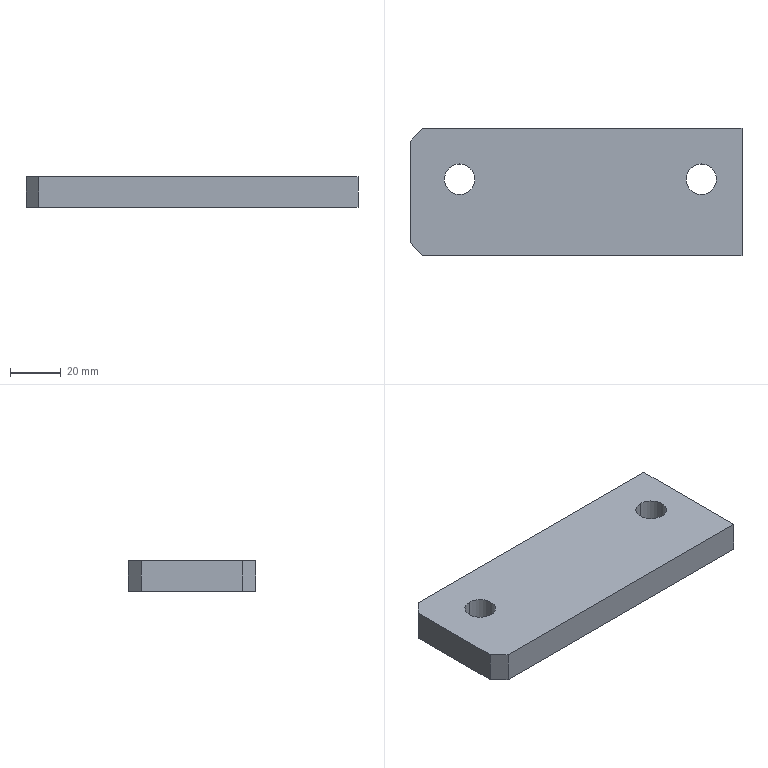Part | STEP file | [13] | 1 solid | 12 faces | box 130.5 x 50 x 12 mm | volume 75286 mm3 | plane 8 | cylinder 4 | commonest cylinder face diameters 12 x4
STEP:
#1=CARTESIAN_POINT('',(114.5,36.,12.));
#2=VERTEX_POINT('',#1);
#3=CARTESIAN_POINT('',(114.5,24.,12.));
#4=VERTEX_POINT('',#3);
#5=CARTESIAN_POINT('',(114.5,30.,12.));
#6=DIRECTION('',(0.,0.,-1.));
#7=DIRECTION('',(0.,-1.,0.));
#8=AXIS2_PLACEMENT_3D('',#5,#6,#7);
#9=CIRCLE('',#8,6.);
#10=EDGE_CURVE('',#2,#4,#9,.T.);
#11=ORIENTED_EDGE('',*,*,#10,.F.);
#12=CARTESIAN_POINT('',(114.5,36.,0.));
#13=VERTEX_POINT('',#12);
#14=CARTESIAN_POINT('',(114.5,36.,12.));
#15=DIRECTION('',(0.,0.,-1.));
#16=VECTOR('',#15,1000.);
#17=LINE('',#14,#16);
#18=EDGE_CURVE('',#2,#13,#17,.T.);
#19=ORIENTED_EDGE('',*,*,#18,.T.);
#20=CARTESIAN_POINT('',(114.5,24.,0.));
#21=VERTEX_POINT('',#20);
#22=CARTESIAN_POINT('',(114.5,30.,0.));
#23=DIRECTION('',(0.,0.,1.));
#24=DIRECTION('',(0.,1.,0.));
#25=AXIS2_PLACEMENT_3D('',#22,#23,#24);
#26=CIRCLE('',#25,6.);
#27=EDGE_CURVE('',#21,#13,#26,.T.);
#28=ORIENTED_EDGE('',*,*,#27,.F.);
#29=CARTESIAN_POINT('',(114.5,24.,12.));
#30=DIRECTION('',(0.,0.,-1.));
#31=VECTOR('',#30,1000.);
#32=LINE('',#29,#31);
#33=EDGE_CURVE('',#4,#21,#32,.T.);
#34=ORIENTED_EDGE('',*,*,#33,.F.);
#35=EDGE_LOOP('',(#11,#19,#28,#34));
#36=FACE_OUTER_BOUND('',#35,.T.);
#37=CARTESIAN_POINT('',(114.5,30.,12.));
#38=DIRECTION('',(0.,0.,-1.));
#39=DIRECTION('',(0.,-1.,0.));
#40=AXIS2_PLACEMENT_3D('',#37,#38,#39);
#41=CYLINDRICAL_SURFACE('',#40,6.);
#42=ADVANCED_FACE('',(#36),#41,.F.);
#43=CARTESIAN_POINT('',(19.5,36.,12.));
#44=VERTEX_POINT('',#43);
#45=CARTESIAN_POINT('',(19.5,24.,12.));
#46=VERTEX_POINT('',#45);
#47=CARTESIAN_POINT('',(19.5,30.,12.));
#48=DIRECTION('',(0.,0.,-1.));
#49=DIRECTION('',(0.,-1.,0.));
#50=AXIS2_PLACEMENT_3D('',#47,#48,#49);
#51=CIRCLE('',#50,6.);
#52=EDGE_CURVE('',#44,#46,#51,.T.);
#53=ORIENTED_EDGE('',*,*,#52,.F.);
#54=CARTESIAN_POINT('',(19.5,36.,0.));
#55=VERTEX_POINT('',#54);
#56=CARTESIAN_POINT('',(19.5,36.,12.));
#57=DIRECTION('',(0.,0.,-1.));
#58=VECTOR('',#57,1000.);
#59=LINE('',#56,#58);
#60=EDGE_CURVE('',#44,#55,#59,.T.);
#61=ORIENTED_EDGE('',*,*,#60,.T.);
#62=CARTESIAN_POINT('',(19.5,24.,0.));
#63=VERTEX_POINT('',#62);
#64=CARTESIAN_POINT('',(19.5,30.,0.));
#65=DIRECTION('',(0.,0.,1.));
#66=DIRECTION('',(0.,1.,0.));
#67=AXIS2_PLACEMENT_3D('',#64,#65,#66);
#68=CIRCLE('',#67,6.);
#69=EDGE_CURVE('',#63,#55,#68,.T.);
#70=ORIENTED_EDGE('',*,*,#69,.F.);
#71=CARTESIAN_POINT('',(19.5,24.,12.));
#72=DIRECTION('',(0.,0.,-1.));
#73=VECTOR('',#72,1000.);
#74=LINE('',#71,#73);
#75=EDGE_CURVE('',#46,#63,#74,.T.);
#76=ORIENTED_EDGE('',*,*,#75,.F.);
#77=EDGE_LOOP('',(#53,#61,#70,#76));
#78=FACE_OUTER_BOUND('',#77,.T.);
#79=CARTESIAN_POINT('',(19.5,30.,12.));
#80=DIRECTION('',(0.,0.,-1.));
#81=DIRECTION('',(0.,-1.,0.));
#82=AXIS2_PLACEMENT_3D('',#79,#80,#81);
#83=CYLINDRICAL_SURFACE('',#82,6.);
#84=ADVANCED_FACE('',(#78),#83,.F.);
#85=CARTESIAN_POINT('',(114.5,30.,12.));
#86=DIRECTION('',(0.,0.,-1.));
#87=DIRECTION('',(0.,-1.,0.));
#88=AXIS2_PLACEMENT_3D('',#85,#86,#87);
#89=CIRCLE('',#88,6.);
#90=EDGE_CURVE('',#4,#2,#89,.T.);
#91=ORIENTED_EDGE('',*,*,#90,.T.);
#92=ORIENTED_EDGE('',*,*,#10,.T.);
#93=EDGE_LOOP('',(#91,#92));
#94=FACE_BOUND('',#93,.T.);
#95=CARTESIAN_POINT('',(19.5,30.,12.));
#96=DIRECTION('',(0.,0.,-1.));
#97=DIRECTION('',(0.,-1.,0.));
#98=AXIS2_PLACEMENT_3D('',#95,#96,#97);
#99=CIRCLE('',#98,6.);
#100=EDGE_CURVE('',#46,#44,#99,.T.);
#101=ORIENTED_EDGE('',*,*,#100,.T.);
#102=ORIENTED_EDGE('',*,*,#52,.T.);
#103=EDGE_LOOP('',(#101,#102));
#104=FACE_BOUND('',#103,.T.);
#105=CARTESIAN_POINT('',(5.,50.,12.));
#106=VERTEX_POINT('',#105);
#107=CARTESIAN_POINT('',(130.5,50.,12.));
#108=VERTEX_POINT('',#107);
#109=CARTESIAN_POINT('',(65.25,50.,12.));
#110=DIRECTION('',(1.,0.,0.));
#111=VECTOR('',#110,1000.);
#112=LINE('',#109,#111);
#113=EDGE_CURVE('',#106,#108,#112,.T.);
#114=ORIENTED_EDGE('',*,*,#113,.F.);
#115=CARTESIAN_POINT('',(0.,45.,12.));
#116=VERTEX_POINT('',#115);
#117=CARTESIAN_POINT('',(22.625,67.625,12.));
#118=DIRECTION('',(-0.7071,-0.7071,0.));
#119=VECTOR('',#118,1000.);
#120=LINE('',#117,#119);
#121=EDGE_CURVE('',#106,#116,#120,.T.);
#122=ORIENTED_EDGE('',*,*,#121,.T.);
#123=CARTESIAN_POINT('',(0.,5.,12.));
#124=VERTEX_POINT('',#123);
#125=CARTESIAN_POINT('',(0.,25.,12.));
#126=DIRECTION('',(0.,1.,0.));
#127=VECTOR('',#126,1000.);
#128=LINE('',#125,#127);
#129=EDGE_CURVE('',#124,#116,#128,.T.);
#130=ORIENTED_EDGE('',*,*,#129,.F.);
#131=CARTESIAN_POINT('',(5.,0.,12.));
#132=VERTEX_POINT('',#131);
#133=CARTESIAN_POINT('',(22.625,-17.625,12.));
#134=DIRECTION('',(0.7071,-0.7071,0.));
#135=VECTOR('',#134,1000.);
#136=LINE('',#133,#135);
#137=EDGE_CURVE('',#124,#132,#136,.T.);
#138=ORIENTED_EDGE('',*,*,#137,.T.);
#139=CARTESIAN_POINT('',(130.5,0.,12.));
#140=VERTEX_POINT('',#139);
#141=CARTESIAN_POINT('',(65.25,0.,12.));
#142=DIRECTION('',(-1.,0.,0.));
#143=VECTOR('',#142,1000.);
#144=LINE('',#141,#143);
#145=EDGE_CURVE('',#140,#132,#144,.T.);
#146=ORIENTED_EDGE('',*,*,#145,.F.);
#147=CARTESIAN_POINT('',(130.5,25.,12.));
#148=DIRECTION('',(0.,-1.,0.));
#149=VECTOR('',#148,1000.);
#150=LINE('',#147,#149);
#151=EDGE_CURVE('',#108,#140,#150,.T.);
#152=ORIENTED_EDGE('',*,*,#151,.F.);
#153=EDGE_LOOP('',(#114,#122,#130,#138,#146,#152));
#154=FACE_OUTER_BOUND('',#153,.T.);
#155=CARTESIAN_POINT('',(65.25,25.,12.));
#156=DIRECTION('',(0.,0.,1.));
#157=DIRECTION('',(1.,0.,0.));
#158=AXIS2_PLACEMENT_3D('',#155,#156,#157);
#159=PLANE('',#158);
#160=ADVANCED_FACE('',(#94,#104,#154),#159,.T.);
#161=ORIENTED_EDGE('',*,*,#145,.T.);
#162=CARTESIAN_POINT('',(5.,0.,0.));
#163=VERTEX_POINT('',#162);
#164=CARTESIAN_POINT('',(5.,0.,0.));
#165=DIRECTION('',(0.,0.,-1.));
#166=VECTOR('',#165,1000.);
#167=LINE('',#164,#166);
#168=EDGE_CURVE('',#132,#163,#167,.T.);
#169=ORIENTED_EDGE('',*,*,#168,.T.);
#170=CARTESIAN_POINT('',(130.5,0.,0.));
#171=VERTEX_POINT('',#170);
#172=CARTESIAN_POINT('',(65.25,0.,0.));
#173=DIRECTION('',(1.,0.,0.));
#174=VECTOR('',#173,1000.);
#175=LINE('',#172,#174);
#176=EDGE_CURVE('',#163,#171,#175,.T.);
#177=ORIENTED_EDGE('',*,*,#176,.T.);
#178=CARTESIAN_POINT('',(130.5,0.,0.));
#179=DIRECTION('',(0.,0.,1.));
#180=VECTOR('',#179,1000.);
#181=LINE('',#178,#180);
#182=EDGE_CURVE('',#171,#140,#181,.T.);
#183=ORIENTED_EDGE('',*,*,#182,.T.);
#184=EDGE_LOOP('',(#161,#169,#177,#183));
#185=FACE_OUTER_BOUND('',#184,.T.);
#186=CARTESIAN_POINT('',(65.25,0.,0.));
#187=DIRECTION('',(0.,-1.,0.));
#188=DIRECTION('',(0.,0.,-1.));
#189=AXIS2_PLACEMENT_3D('',#186,#187,#188);
#190=PLANE('',#189);
#191=ADVANCED_FACE('',(#185),#190,.T.);
#192=ORIENTED_EDGE('',*,*,#129,.T.);
#193=CARTESIAN_POINT('',(0.,45.,0.));
#194=VERTEX_POINT('',#193);
#195=CARTESIAN_POINT('',(0.,45.,0.));
#196=DIRECTION('',(0.,0.,-1.));
#197=VECTOR('',#196,1000.);
#198=LINE('',#195,#197);
#199=EDGE_CURVE('',#116,#194,#198,.T.);
#200=ORIENTED_EDGE('',*,*,#199,.T.);
#201=CARTESIAN_POINT('',(0.,5.,0.));
#202=VERTEX_POINT('',#201);
#203=CARTESIAN_POINT('',(0.,25.,0.));
#204=DIRECTION('',(0.,-1.,0.));
#205=VECTOR('',#204,1000.);
#206=LINE('',#203,#205);
#207=EDGE_CURVE('',#194,#202,#206,.T.);
#208=ORIENTED_EDGE('',*,*,#207,.T.);
#209=CARTESIAN_POINT('',(0.,5.,0.));
#210=DIRECTION('',(0.,0.,1.));
#211=VECTOR('',#210,1000.);
#212=LINE('',#209,#211);
#213=EDGE_CURVE('',#202,#124,#212,.T.);
#214=ORIENTED_EDGE('',*,*,#213,.T.);
#215=EDGE_LOOP('',(#192,#200,#208,#214));
#216=FACE_OUTER_BOUND('',#215,.T.);
#217=CARTESIAN_POINT('',(0.,25.,0.));
#218=DIRECTION('',(-1.,0.,0.));
#219=DIRECTION('',(0.,0.,1.));
#220=AXIS2_PLACEMENT_3D('',#217,#218,#219);
#221=PLANE('',#220);
#222=ADVANCED_FACE('',(#216),#221,.T.);
#223=CARTESIAN_POINT('',(130.5,50.,0.));
#224=VERTEX_POINT('',#223);
#225=CARTESIAN_POINT('',(5.,50.,0.));
#226=VERTEX_POINT('',#225);
#227=CARTESIAN_POINT('',(65.25,50.,0.));
#228=DIRECTION('',(-1.,0.,0.));
#229=VECTOR('',#228,1000.);
#230=LINE('',#227,#229);
#231=EDGE_CURVE('',#224,#226,#230,.T.);
#232=ORIENTED_EDGE('',*,*,#231,.T.);
#233=CARTESIAN_POINT('',(5.,50.,0.));
#234=DIRECTION('',(0.,0.,1.));
#235=VECTOR('',#234,1000.);
#236=LINE('',#233,#235);
#237=EDGE_CURVE('',#226,#106,#236,.T.);
#238=ORIENTED_EDGE('',*,*,#237,.T.);
#239=ORIENTED_EDGE('',*,*,#113,.T.);
#240=CARTESIAN_POINT('',(130.5,50.,0.));
#241=DIRECTION('',(0.,0.,1.));
#242=VECTOR('',#241,1000.);
#243=LINE('',#240,#242);
#244=EDGE_CURVE('',#224,#108,#243,.T.);
#245=ORIENTED_EDGE('',*,*,#244,.F.);
#246=EDGE_LOOP('',(#232,#238,#239,#245));
#247=FACE_OUTER_BOUND('',#246,.T.);
#248=CARTESIAN_POINT('',(65.25,50.,0.));
#249=DIRECTION('',(0.,1.,0.));
#250=DIRECTION('',(0.,0.,1.));
#251=AXIS2_PLACEMENT_3D('',#248,#249,#250);
#252=PLANE('',#251);
#253=ADVANCED_FACE('',(#247),#252,.T.);
#254=ORIENTED_EDGE('',*,*,#69,.T.);
#255=CARTESIAN_POINT('',(19.5,30.,0.));
#256=DIRECTION('',(0.,0.,1.));
#257=DIRECTION('',(0.,1.,0.));
#258=AXIS2_PLACEMENT_3D('',#255,#256,#257);
#259=CIRCLE('',#258,6.);
#260=EDGE_CURVE('',#55,#63,#259,.T.);
#261=ORIENTED_EDGE('',*,*,#260,.T.);
#262=EDGE_LOOP('',(#254,#261));
#263=FACE_BOUND('',#262,.T.);
#264=ORIENTED_EDGE('',*,*,#207,.F.);
#265=CARTESIAN_POINT('',(22.625,67.625,0.));
#266=DIRECTION('',(0.7071,0.7071,0.));
#267=VECTOR('',#266,1000.);
#268=LINE('',#265,#267);
#269=EDGE_CURVE('',#194,#226,#268,.T.);
#270=ORIENTED_EDGE('',*,*,#269,.T.);
#271=ORIENTED_EDGE('',*,*,#231,.F.);
#272=CARTESIAN_POINT('',(130.5,25.,0.));
#273=DIRECTION('',(0.,1.,0.));
#274=VECTOR('',#273,1000.);
#275=LINE('',#272,#274);
#276=EDGE_CURVE('',#171,#224,#275,.T.);
#277=ORIENTED_EDGE('',*,*,#276,.F.);
#278=ORIENTED_EDGE('',*,*,#176,.F.);
#279=CARTESIAN_POINT('',(22.625,-17.625,0.));
#280=DIRECTION('',(-0.7071,0.7071,0.));
#281=VECTOR('',#280,1000.);
#282=LINE('',#279,#281);
#283=EDGE_CURVE('',#163,#202,#282,.T.);
#284=ORIENTED_EDGE('',*,*,#283,.T.);
#285=EDGE_LOOP('',(#264,#270,#271,#277,#278,#284));
#286=FACE_OUTER_BOUND('',#285,.T.);
#287=ORIENTED_EDGE('',*,*,#27,.T.);
#288=CARTESIAN_POINT('',(114.5,30.,0.));
#289=DIRECTION('',(0.,0.,1.));
#290=DIRECTION('',(0.,1.,0.));
#291=AXIS2_PLACEMENT_3D('',#288,#289,#290);
#292=CIRCLE('',#291,6.);
#293=EDGE_CURVE('',#13,#21,#292,.T.);
#294=ORIENTED_EDGE('',*,*,#293,.T.);
#295=EDGE_LOOP('',(#287,#294));
#296=FACE_BOUND('',#295,.T.);
#297=CARTESIAN_POINT('',(65.25,25.,0.));
#298=DIRECTION('',(0.,0.,-1.));
#299=DIRECTION('',(-1.,0.,0.));
#300=AXIS2_PLACEMENT_3D('',#297,#298,#299);
#301=PLANE('',#300);
#302=ADVANCED_FACE('',(#263,#286,#296),#301,.T.);
#303=ORIENTED_EDGE('',*,*,#276,.T.);
#304=ORIENTED_EDGE('',*,*,#244,.T.);
#305=ORIENTED_EDGE('',*,*,#151,.T.);
#306=ORIENTED_EDGE('',*,*,#182,.F.);
#307=EDGE_LOOP('',(#303,#304,#305,#306));
#308=FACE_OUTER_BOUND('',#307,.T.);
#309=CARTESIAN_POINT('',(130.5,25.,0.));
#310=DIRECTION('',(1.,0.,0.));
#311=DIRECTION('',(0.,0.,-1.));
#312=AXIS2_PLACEMENT_3D('',#309,#310,#311);
#313=PLANE('',#312);
#314=ADVANCED_FACE('',(#308),#313,.T.);
#315=ORIENTED_EDGE('',*,*,#60,.F.);
#316=ORIENTED_EDGE('',*,*,#100,.F.);
#317=ORIENTED_EDGE('',*,*,#75,.T.);
#318=ORIENTED_EDGE('',*,*,#260,.F.);
#319=EDGE_LOOP('',(#315,#316,#317,#318));
#320=FACE_OUTER_BOUND('',#319,.T.);
#321=CARTESIAN_POINT('',(19.5,30.,12.));
#322=DIRECTION('',(0.,0.,-1.));
#323=DIRECTION('',(0.,-1.,0.));
#324=AXIS2_PLACEMENT_3D('',#321,#322,#323);
#325=CYLINDRICAL_SURFACE('',#324,6.);
#326=ADVANCED_FACE('',(#320),#325,.F.);
#327=ORIENTED_EDGE('',*,*,#18,.F.);
#328=ORIENTED_EDGE('',*,*,#90,.F.);
#329=ORIENTED_EDGE('',*,*,#33,.T.);
#330=ORIENTED_EDGE('',*,*,#293,.F.);
#331=EDGE_LOOP('',(#327,#328,#329,#330));
#332=FACE_OUTER_BOUND('',#331,.T.);
#333=CARTESIAN_POINT('',(114.5,30.,12.));
#334=DIRECTION('',(0.,0.,-1.));
#335=DIRECTION('',(0.,-1.,0.));
#336=AXIS2_PLACEMENT_3D('',#333,#334,#335);
#337=CYLINDRICAL_SURFACE('',#336,6.);
#338=ADVANCED_FACE('',(#332),#337,.F.);
#339=ORIENTED_EDGE('',*,*,#283,.F.);
#340=ORIENTED_EDGE('',*,*,#168,.F.);
#341=ORIENTED_EDGE('',*,*,#137,.F.);
#342=ORIENTED_EDGE('',*,*,#213,.F.);
#343=EDGE_LOOP('',(#339,#340,#341,#342));
#344=FACE_OUTER_BOUND('',#343,.T.);
#345=CARTESIAN_POINT('',(0.,5.,0.));
#346=DIRECTION('',(0.7071,0.7071,0.));
#347=DIRECTION('',(0.,0.,1.));
#348=AXIS2_PLACEMENT_3D('',#345,#346,#347);
#349=PLANE('',#348);
#350=ADVANCED_FACE('',(#344),#349,.F.);
#351=ORIENTED_EDGE('',*,*,#269,.F.);
#352=ORIENTED_EDGE('',*,*,#199,.F.);
#353=ORIENTED_EDGE('',*,*,#121,.F.);
#354=ORIENTED_EDGE('',*,*,#237,.F.);
#355=EDGE_LOOP('',(#351,#352,#353,#354));
#356=FACE_OUTER_BOUND('',#355,.T.);
#357=CARTESIAN_POINT('',(5.,50.,0.));
#358=DIRECTION('',(0.7071,-0.7071,0.));
#359=DIRECTION('',(0.,0.,1.));
#360=AXIS2_PLACEMENT_3D('',#357,#358,#359);
#361=PLANE('',#360);
#362=ADVANCED_FACE('',(#356),#361,.F.);
#363=CLOSED_SHELL('',(#42,#84,#160,#191,#222,#253,#302,#314,#326,#338,#350,#362));
#364=MANIFOLD_SOLID_BREP('',#363);
#365=CARTESIAN_POINT('',(0.,0.,0.));
#366=DIRECTION('',(0.,0.,1.));
#367=DIRECTION('',(1.,0.,0.));
#368=AXIS2_PLACEMENT_3D('',#365,#366,#367);
#369=(LENGTH_UNIT()NAMED_UNIT(*)SI_UNIT(.MILLI.,.METRE.));
#370=UNCERTAINTY_MEASURE_WITH_UNIT(LENGTH_MEASURE(0.00001),#369,'','');
#371=(NAMED_UNIT(*)PLANE_ANGLE_UNIT()SI_UNIT($,.RADIAN.));
#372=(NAMED_UNIT(*)SI_UNIT($,.STERADIAN.)SOLID_ANGLE_UNIT());
#373=(GEOMETRIC_REPRESENTATION_CONTEXT(3)GLOBAL_UNCERTAINTY_ASSIGNED_CONTEXT((#370))GLOBAL_UNIT_ASSIGNED_CONTEXT((#369,#371,#372))REPRESENTATION_CONTEXT('',''));
#374=ADVANCED_BREP_SHAPE_REPRESENTATION('',(#364,#368),#373);